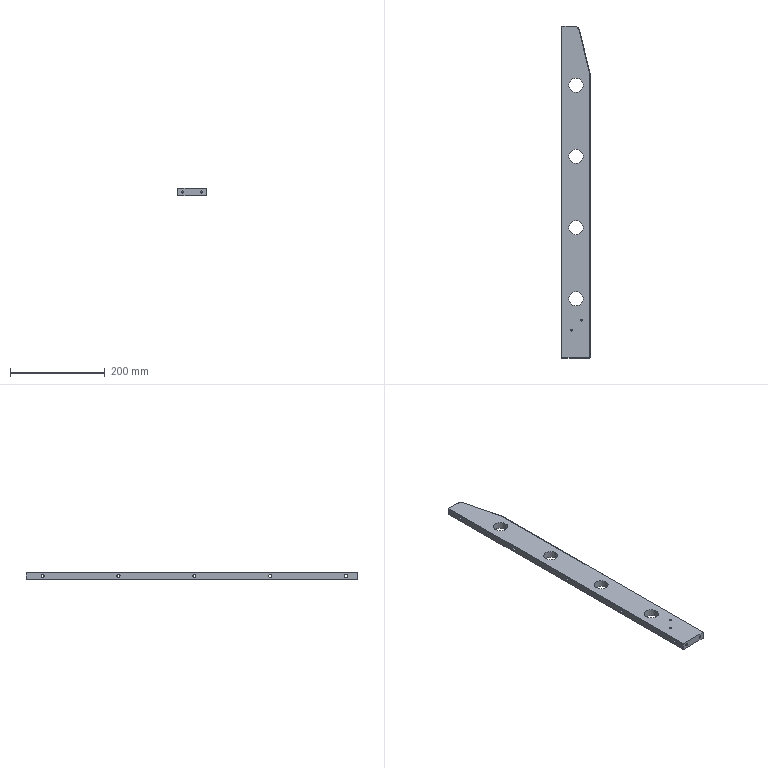Part | STEP file | 1 solid | 41 faces | box 60 x 700 x 15 mm | volume 546170 mm3 | cylinder 25 | plane 12 | spline 2 | cone 2 | commonest cylinder face diameters 2 x6 6.5 x5 10 x5 30 x4 4.2 x2 5 x2